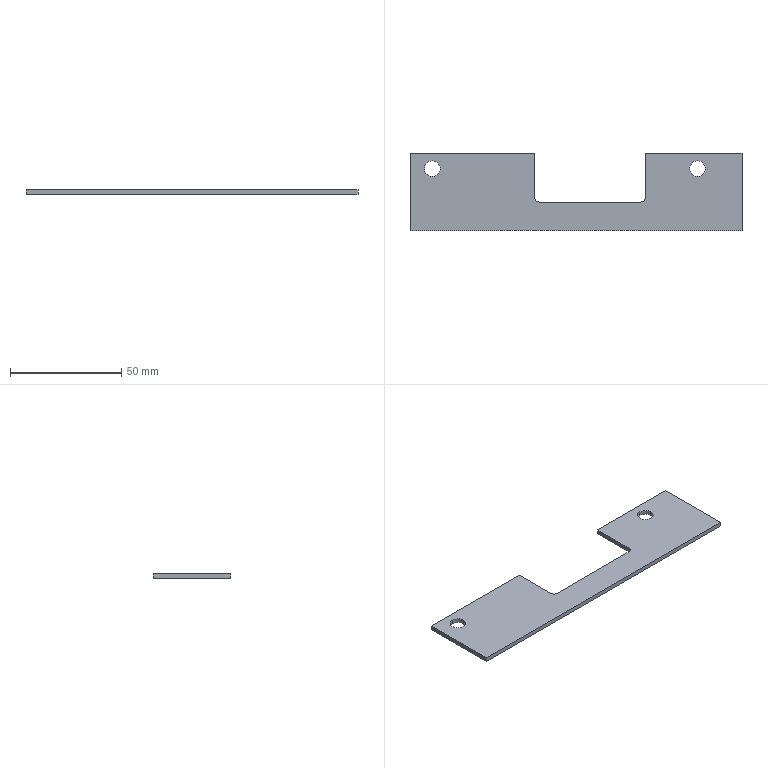Part | STEP file | 1_id638_x_t | 1 solid | 16 faces | box 149 x 35 x 2 mm | volume 8095 mm3 | plane 10 | cylinder 6 | commonest cylinder face diameters 7 x4 4 x2
STEP:
#1=CARTESIAN_POINT('',(0.,0.,0.));
#2=DIRECTION('',(0.,0.,1.));
#3=DIRECTION('',(1.,0.,0.));
#4=AXIS2_PLACEMENT_3D('',#1,#2,#3);
#5=CARTESIAN_POINT('',(650.204,237.475,-88.));
#6=VERTEX_POINT('',#5);
#7=CARTESIAN_POINT('',(648.204,235.475,-88.));
#8=VERTEX_POINT('',#7);
#9=CARTESIAN_POINT('',(648.204,237.475,-88.));
#10=DIRECTION('',(0.,0.,-1.));
#11=DIRECTION('',(1.,0.,0.));
#12=AXIS2_PLACEMENT_3D('',#9,#10,#11);
#13=CIRCLE('',#12,2.);
#14=CARTESIAN_POINT('',(499.55,257.475,-88.));
#15=DIRECTION('',(0.,0.,1.));
#16=DIRECTION('',(0.,1.,0.));
#17=AXIS2_PLACEMENT_3D('',#14,#15,#16);
#18=PLANE('',#17);
#19=CARTESIAN_POINT('',(-20.,-150.654));
#20=CARTESIAN_POINT('',(-23.464,-150.654));
#21=CARTESIAN_POINT('',(-21.732,-147.654));
#22=CARTESIAN_POINT('',(-20.,-144.654));
#23=CARTESIAN_POINT('',(-18.268,-147.654));
#24=CARTESIAN_POINT('',(-16.536,-150.654));
#25=CARTESIAN_POINT('',(-20.,-150.654));
#26=(BOUNDED_CURVE()B_SPLINE_CURVE(2,(#19,#20,#21,#22,#23,#24,#25),.UNSPECIFIED.,.T.,.F.)B_SPLINE_CURVE_WITH_KNOTS((1,2,2,2,2,1),(-2.094,0.,2.094,4.189,6.283,8.378),.UNSPECIFIED.)CURVE()GEOMETRIC_REPRESENTATION_ITEM()RATIONAL_B_SPLINE_CURVE((1.,0.5,1.,0.5,1.,0.5,1.))REPRESENTATION_ITEM(''));
#27=(GEOMETRIC_REPRESENTATION_CONTEXT(2)PARAMETRIC_REPRESENTATION_CONTEXT()REPRESENTATION_CONTEXT('',''));
#28=DEFINITIONAL_REPRESENTATION('',(#26),#27);
#29=PCURVE('',#18,#28);
#30=CARTESIAN_POINT('',(648.204,237.475,-92.));
#31=DIRECTION('',(0.,0.,-1.));
#32=DIRECTION('',(0.,1.,0.));
#33=AXIS2_PLACEMENT_3D('',#30,#31,#32);
#34=CYLINDRICAL_SURFACE('',#33,2.);
#35=CARTESIAN_POINT('',(1.571,-4.));
#36=DIRECTION('',(1.,0.));
#37=VECTOR('',#36,1.);
#38=LINE('',#35,#37);
#39=(GEOMETRIC_REPRESENTATION_CONTEXT(2)PARAMETRIC_REPRESENTATION_CONTEXT()REPRESENTATION_CONTEXT('',''));
#40=DEFINITIONAL_REPRESENTATION('',(#38),#39);
#41=PCURVE('',#34,#40);
#42=SURFACE_CURVE('',#13,(#29,#41),.PCURVE_S1.);
#43=EDGE_CURVE('',#6,#8,#42,.T.);
#44=ORIENTED_EDGE('',*,*,#43,.T.);
#45=CARTESIAN_POINT('',(602.55,235.475,-88.));
#46=VERTEX_POINT('',#45);
#47=CARTESIAN_POINT('',(648.204,235.475,-88.));
#48=DIRECTION('',(-1.,0.,0.));
#49=VECTOR('',#48,1.);
#50=LINE('',#47,#49);
#51=CARTESIAN_POINT('',(-22.,-148.654));
#52=DIRECTION('',(0.,1.));
#53=VECTOR('',#52,1.);
#54=LINE('',#51,#53);
#55=(GEOMETRIC_REPRESENTATION_CONTEXT(2)PARAMETRIC_REPRESENTATION_CONTEXT()REPRESENTATION_CONTEXT('',''));
#56=DEFINITIONAL_REPRESENTATION('',(#54),#55);
#57=PCURVE('',#18,#56);
#58=CARTESIAN_POINT('',(629.402,235.475,-92.));
#59=DIRECTION('',(0.,-1.,0.));
#60=DIRECTION('',(0.,0.,-1.));
#61=AXIS2_PLACEMENT_3D('',#58,#59,#60);
#62=PLANE('',#61);
#63=CARTESIAN_POINT('',(-4.,18.802));
#64=DIRECTION('',(0.,-1.));
#65=VECTOR('',#64,1.);
#66=LINE('',#63,#65);
#67=(GEOMETRIC_REPRESENTATION_CONTEXT(2)PARAMETRIC_REPRESENTATION_CONTEXT()REPRESENTATION_CONTEXT('',''));
#68=DEFINITIONAL_REPRESENTATION('',(#66),#67);
#69=PCURVE('',#62,#68);
#70=SURFACE_CURVE('',#50,(#57,#69),.PCURVE_S1.);
#71=EDGE_CURVE('',#8,#46,#70,.T.);
#72=ORIENTED_EDGE('',*,*,#71,.T.);
#73=CARTESIAN_POINT('',(600.55,237.475,-88.));
#74=VERTEX_POINT('',#73);
#75=CARTESIAN_POINT('',(602.55,237.475,-88.));
#76=DIRECTION('',(0.,0.,-1.));
#77=DIRECTION('',(0.,-1.,0.));
#78=AXIS2_PLACEMENT_3D('',#75,#76,#77);
#79=CIRCLE('',#78,2.);
#80=CARTESIAN_POINT('',(-22.,-103.));
#81=CARTESIAN_POINT('',(-22.,-99.536));
#82=CARTESIAN_POINT('',(-19.,-101.268));
#83=CARTESIAN_POINT('',(-16.,-103.));
#84=CARTESIAN_POINT('',(-19.,-104.732));
#85=CARTESIAN_POINT('',(-22.,-106.464));
#86=CARTESIAN_POINT('',(-22.,-103.));
#87=(BOUNDED_CURVE()B_SPLINE_CURVE(2,(#80,#81,#82,#83,#84,#85,#86),.UNSPECIFIED.,.T.,.F.)B_SPLINE_CURVE_WITH_KNOTS((1,2,2,2,2,1),(-2.094,0.,2.094,4.189,6.283,8.378),.UNSPECIFIED.)CURVE()GEOMETRIC_REPRESENTATION_ITEM()RATIONAL_B_SPLINE_CURVE((1.,0.5,1.,0.5,1.,0.5,1.))REPRESENTATION_ITEM(''));
#88=(GEOMETRIC_REPRESENTATION_CONTEXT(2)PARAMETRIC_REPRESENTATION_CONTEXT()REPRESENTATION_CONTEXT('',''));
#89=DEFINITIONAL_REPRESENTATION('',(#87),#88);
#90=PCURVE('',#18,#89);
#91=CARTESIAN_POINT('',(602.55,237.475,-92.));
#92=DIRECTION('',(0.,0.,-1.));
#93=DIRECTION('',(0.,1.,0.));
#94=AXIS2_PLACEMENT_3D('',#91,#92,#93);
#95=CYLINDRICAL_SURFACE('',#94,2.);
#96=CARTESIAN_POINT('',(3.142,-4.));
#97=DIRECTION('',(1.,0.));
#98=VECTOR('',#97,1.);
#99=LINE('',#96,#98);
#100=(GEOMETRIC_REPRESENTATION_CONTEXT(2)PARAMETRIC_REPRESENTATION_CONTEXT()REPRESENTATION_CONTEXT('',''));
#101=DEFINITIONAL_REPRESENTATION('',(#99),#100);
#102=PCURVE('',#95,#101);
#103=SURFACE_CURVE('',#79,(#90,#102),.PCURVE_S1.);
#104=EDGE_CURVE('',#46,#74,#103,.T.);
#105=ORIENTED_EDGE('',*,*,#104,.T.);
#106=CARTESIAN_POINT('',(600.55,257.475,-88.));
#107=VERTEX_POINT('',#106);
#108=CARTESIAN_POINT('',(600.55,237.475,-88.));
#109=DIRECTION('',(0.,1.,0.));
#110=VECTOR('',#109,1.);
#111=LINE('',#108,#110);
#112=CARTESIAN_POINT('',(-20.,-101.));
#113=DIRECTION('',(1.,0.));
#114=VECTOR('',#113,1.);
#115=LINE('',#112,#114);
#116=(GEOMETRIC_REPRESENTATION_CONTEXT(2)PARAMETRIC_REPRESENTATION_CONTEXT()REPRESENTATION_CONTEXT('',''));
#117=DEFINITIONAL_REPRESENTATION('',(#115),#116);
#118=PCURVE('',#18,#117);
#119=CARTESIAN_POINT('',(600.55,253.588,-92.));
#120=DIRECTION('',(-1.,0.,0.));
#121=DIRECTION('',(0.,0.,-1.));
#122=AXIS2_PLACEMENT_3D('',#119,#120,#121);
#123=PLANE('',#122);
#124=CARTESIAN_POINT('',(-4.,16.113));
#125=DIRECTION('',(0.,-1.));
#126=VECTOR('',#125,1.);
#127=LINE('',#124,#126);
#128=(GEOMETRIC_REPRESENTATION_CONTEXT(2)PARAMETRIC_REPRESENTATION_CONTEXT()REPRESENTATION_CONTEXT('',''));
#129=DEFINITIONAL_REPRESENTATION('',(#127),#128);
#130=PCURVE('',#123,#129);
#131=SURFACE_CURVE('',#111,(#118,#130),.PCURVE_S1.);
#132=EDGE_CURVE('',#74,#107,#131,.T.);
#133=ORIENTED_EDGE('',*,*,#132,.T.);
#134=CARTESIAN_POINT('',(544.55,257.475,-88.));
#135=VERTEX_POINT('',#134);
#136=CARTESIAN_POINT('',(544.55,257.475,-88.));
#137=DIRECTION('',(1.,0.,0.));
#138=VECTOR('',#137,1.);
#139=LINE('',#136,#138);
#140=CARTESIAN_POINT('',(0.,-45.));
#141=DIRECTION('',(0.,-1.));
#142=VECTOR('',#141,1.);
#143=LINE('',#140,#142);
#144=(GEOMETRIC_REPRESENTATION_CONTEXT(2)PARAMETRIC_REPRESENTATION_CONTEXT()REPRESENTATION_CONTEXT('',''));
#145=DEFINITIONAL_REPRESENTATION('',(#143),#144);
#146=PCURVE('',#18,#145);
#147=CARTESIAN_POINT('',(744.55,257.475,-88.));
#148=DIRECTION('',(0.,-1.,0.));
#149=DIRECTION('',(1.,0.,0.));
#150=AXIS2_PLACEMENT_3D('',#147,#148,#149);
#151=PLANE('',#150);
#152=CARTESIAN_POINT('',(-200.,0.));
#153=DIRECTION('',(1.,0.));
#154=VECTOR('',#153,1.);
#155=LINE('',#152,#154);
#156=(GEOMETRIC_REPRESENTATION_CONTEXT(2)PARAMETRIC_REPRESENTATION_CONTEXT()REPRESENTATION_CONTEXT('',''));
#157=DEFINITIONAL_REPRESENTATION('',(#155),#156);
#158=PCURVE('',#151,#157);
#159=SURFACE_CURVE('',#139,(#146,#158),.PCURVE_S1.);
#160=EDGE_CURVE('',#135,#107,#159,.T.);
#161=ORIENTED_EDGE('',*,*,#160,.F.);
#162=CARTESIAN_POINT('',(544.55,222.475,-88.));
#163=VERTEX_POINT('',#162);
#164=CARTESIAN_POINT('',(544.55,222.475,-88.));
#165=DIRECTION('',(0.,1.,0.));
#166=VECTOR('',#165,1.);
#167=LINE('',#164,#166);
#168=CARTESIAN_POINT('',(-35.,-45.));
#169=DIRECTION('',(1.,0.));
#170=VECTOR('',#169,1.);
#171=LINE('',#168,#170);
#172=(GEOMETRIC_REPRESENTATION_CONTEXT(2)PARAMETRIC_REPRESENTATION_CONTEXT()REPRESENTATION_CONTEXT('',''));
#173=DEFINITIONAL_REPRESENTATION('',(#171),#172);
#174=PCURVE('',#18,#173);
#175=CARTESIAN_POINT('',(544.55,257.475,-88.));
#176=DIRECTION('',(1.,0.,0.));
#177=DIRECTION('',(0.,0.,1.));
#178=AXIS2_PLACEMENT_3D('',#175,#176,#177);
#179=PLANE('',#178);
#180=CARTESIAN_POINT('',(0.,35.));
#181=DIRECTION('',(0.,-1.));
#182=VECTOR('',#181,1.);
#183=LINE('',#180,#182);
#184=(GEOMETRIC_REPRESENTATION_CONTEXT(2)PARAMETRIC_REPRESENTATION_CONTEXT()REPRESENTATION_CONTEXT('',''));
#185=DEFINITIONAL_REPRESENTATION('',(#183),#184);
#186=PCURVE('',#179,#185);
#187=SURFACE_CURVE('',#167,(#174,#186),.PCURVE_S1.);
#188=EDGE_CURVE('',#163,#135,#187,.T.);
#189=ORIENTED_EDGE('',*,*,#188,.F.);
#190=CARTESIAN_POINT('',(693.55,222.475,-88.));
#191=VERTEX_POINT('',#190);
#192=CARTESIAN_POINT('',(693.55,222.475,-88.));
#193=DIRECTION('',(-1.,0.,0.));
#194=VECTOR('',#193,1.);
#195=LINE('',#192,#194);
#196=CARTESIAN_POINT('',(-35.,-194.));
#197=DIRECTION('',(0.,1.));
#198=VECTOR('',#197,1.);
#199=LINE('',#196,#198);
#200=(GEOMETRIC_REPRESENTATION_CONTEXT(2)PARAMETRIC_REPRESENTATION_CONTEXT()REPRESENTATION_CONTEXT('',''));
#201=DEFINITIONAL_REPRESENTATION('',(#199),#200);
#202=PCURVE('',#18,#201);
#203=CARTESIAN_POINT('',(629.402,222.475,-52.5));
#204=DIRECTION('',(0.,-1.,0.));
#205=DIRECTION('',(0.,0.,-1.));
#206=AXIS2_PLACEMENT_3D('',#203,#204,#205);
#207=PLANE('',#206);
#208=CARTESIAN_POINT('',(35.5,64.148));
#209=DIRECTION('',(0.,-1.));
#210=VECTOR('',#209,1.);
#211=LINE('',#208,#210);
#212=(GEOMETRIC_REPRESENTATION_CONTEXT(2)PARAMETRIC_REPRESENTATION_CONTEXT()REPRESENTATION_CONTEXT('',''));
#213=DEFINITIONAL_REPRESENTATION('',(#211),#212);
#214=PCURVE('',#207,#213);
#215=SURFACE_CURVE('',#195,(#202,#214),.PCURVE_S1.);
#216=EDGE_CURVE('',#191,#163,#215,.T.);
#217=ORIENTED_EDGE('',*,*,#216,.F.);
#218=CARTESIAN_POINT('',(693.55,257.475,-88.));
#219=VERTEX_POINT('',#218);
#220=CARTESIAN_POINT('',(693.55,257.475,-88.));
#221=DIRECTION('',(0.,-1.,0.));
#222=VECTOR('',#221,1.);
#223=LINE('',#220,#222);
#224=CARTESIAN_POINT('',(0.,-194.));
#225=DIRECTION('',(-1.,0.));
#226=VECTOR('',#225,1.);
#227=LINE('',#224,#226);
#228=(GEOMETRIC_REPRESENTATION_CONTEXT(2)PARAMETRIC_REPRESENTATION_CONTEXT()REPRESENTATION_CONTEXT('',''));
#229=DEFINITIONAL_REPRESENTATION('',(#227),#228);
#230=PCURVE('',#18,#229);
#231=CARTESIAN_POINT('',(693.55,212.475,-88.));
#232=DIRECTION('',(-1.,0.,0.));
#233=DIRECTION('',(0.,0.,-1.));
#234=AXIS2_PLACEMENT_3D('',#231,#232,#233);
#235=PLANE('',#234);
#236=CARTESIAN_POINT('',(0.,-45.));
#237=DIRECTION('',(0.,1.));
#238=VECTOR('',#237,1.);
#239=LINE('',#236,#238);
#240=(GEOMETRIC_REPRESENTATION_CONTEXT(2)PARAMETRIC_REPRESENTATION_CONTEXT()REPRESENTATION_CONTEXT('',''));
#241=DEFINITIONAL_REPRESENTATION('',(#239),#240);
#242=PCURVE('',#235,#241);
#243=SURFACE_CURVE('',#223,(#230,#242),.PCURVE_S1.);
#244=EDGE_CURVE('',#219,#191,#243,.T.);
#245=ORIENTED_EDGE('',*,*,#244,.F.);
#246=CARTESIAN_POINT('',(650.204,257.475,-88.));
#247=VERTEX_POINT('',#246);
#248=CARTESIAN_POINT('',(650.204,257.475,-88.));
#249=DIRECTION('',(1.,0.,0.));
#250=VECTOR('',#249,1.);
#251=LINE('',#248,#250);
#252=CARTESIAN_POINT('',(0.,-150.654));
#253=DIRECTION('',(0.,-1.));
#254=VECTOR('',#253,1.);
#255=LINE('',#252,#254);
#256=(GEOMETRIC_REPRESENTATION_CONTEXT(2)PARAMETRIC_REPRESENTATION_CONTEXT()REPRESENTATION_CONTEXT('',''));
#257=DEFINITIONAL_REPRESENTATION('',(#255),#256);
#258=PCURVE('',#18,#257);
#259=CARTESIAN_POINT('',(744.55,257.475,-88.));
#260=DIRECTION('',(0.,-1.,0.));
#261=DIRECTION('',(1.,0.,0.));
#262=AXIS2_PLACEMENT_3D('',#259,#260,#261);
#263=PLANE('',#262);
#264=CARTESIAN_POINT('',(-94.346,0.));
#265=DIRECTION('',(1.,0.));
#266=VECTOR('',#265,1.);
#267=LINE('',#264,#266);
#268=(GEOMETRIC_REPRESENTATION_CONTEXT(2)PARAMETRIC_REPRESENTATION_CONTEXT()REPRESENTATION_CONTEXT('',''));
#269=DEFINITIONAL_REPRESENTATION('',(#267),#268);
#270=PCURVE('',#263,#269);
#271=SURFACE_CURVE('',#251,(#258,#270),.PCURVE_S1.);
#272=EDGE_CURVE('',#247,#219,#271,.T.);
#273=ORIENTED_EDGE('',*,*,#272,.F.);
#274=CARTESIAN_POINT('',(650.204,257.475,-88.));
#275=DIRECTION('',(0.,-1.,0.));
#276=VECTOR('',#275,1.);
#277=LINE('',#274,#276);
#278=CARTESIAN_POINT('',(0.,-150.654));
#279=DIRECTION('',(-1.,0.));
#280=VECTOR('',#279,1.);
#281=LINE('',#278,#280);
#282=(GEOMETRIC_REPRESENTATION_CONTEXT(2)PARAMETRIC_REPRESENTATION_CONTEXT()REPRESENTATION_CONTEXT('',''));
#283=DEFINITIONAL_REPRESENTATION('',(#281),#282);
#284=PCURVE('',#18,#283);
#285=CARTESIAN_POINT('',(650.204,253.588,-92.));
#286=DIRECTION('',(1.,0.,0.));
#287=DIRECTION('',(0.,0.,1.));
#288=AXIS2_PLACEMENT_3D('',#285,#286,#287);
#289=PLANE('',#288);
#290=CARTESIAN_POINT('',(4.,-3.888));
#291=DIRECTION('',(0.,1.));
#292=VECTOR('',#291,1.);
#293=LINE('',#290,#292);
#294=(GEOMETRIC_REPRESENTATION_CONTEXT(2)PARAMETRIC_REPRESENTATION_CONTEXT()REPRESENTATION_CONTEXT('',''));
#295=DEFINITIONAL_REPRESENTATION('',(#293),#294);
#296=PCURVE('',#289,#295);
#297=SURFACE_CURVE('',#277,(#284,#296),.PCURVE_S1.);
#298=EDGE_CURVE('',#247,#6,#297,.T.);
#299=ORIENTED_EDGE('',*,*,#298,.T.);
#300=EDGE_LOOP('',(#44,#72,#105,#133,#161,#189,#217,#245,#273,#299));
#301=FACE_BOUND('',#300,.T.);
#302=CARTESIAN_POINT('',(673.55,246.975,-88.));
#303=VERTEX_POINT('',#302);
#304=CARTESIAN_POINT('',(673.55,253.975,-88.));
#305=VERTEX_POINT('',#304);
#306=CARTESIAN_POINT('',(673.55,250.475,-88.));
#307=DIRECTION('',(0.,0.,-1.));
#308=DIRECTION('',(0.,-1.,0.));
#309=AXIS2_PLACEMENT_3D('',#306,#307,#308);
#310=CIRCLE('',#309,3.5);
#311=CARTESIAN_POINT('',(-10.5,-174.));
#312=CARTESIAN_POINT('',(-10.5,-167.938));
#313=CARTESIAN_POINT('',(-5.25,-170.969));
#314=CARTESIAN_POINT('',(0.,-174.));
#315=CARTESIAN_POINT('',(-5.25,-177.031));
#316=CARTESIAN_POINT('',(-10.5,-180.062));
#317=CARTESIAN_POINT('',(-10.5,-174.));
#318=(BOUNDED_CURVE()B_SPLINE_CURVE(2,(#311,#312,#313,#314,#315,#316,#317),.UNSPECIFIED.,.T.,.F.)B_SPLINE_CURVE_WITH_KNOTS((1,2,2,2,2,1),(-2.094,0.,2.094,4.189,6.283,8.378),.UNSPECIFIED.)CURVE()GEOMETRIC_REPRESENTATION_ITEM()RATIONAL_B_SPLINE_CURVE((1.,0.5,1.,0.5,1.,0.5,1.))REPRESENTATION_ITEM(''));
#319=(GEOMETRIC_REPRESENTATION_CONTEXT(2)PARAMETRIC_REPRESENTATION_CONTEXT()REPRESENTATION_CONTEXT('',''));
#320=DEFINITIONAL_REPRESENTATION('',(#318),#319);
#321=PCURVE('',#18,#320);
#322=CARTESIAN_POINT('',(673.55,250.475,-88.));
#323=DIRECTION('',(0.,0.,-1.));
#324=DIRECTION('',(0.,-1.,0.));
#325=AXIS2_PLACEMENT_3D('',#322,#323,#324);
#326=CYLINDRICAL_SURFACE('',#325,3.5);
#327=CARTESIAN_POINT('',(0.,0.));
#328=DIRECTION('',(1.,0.));
#329=VECTOR('',#328,1.);
#330=LINE('',#327,#329);
#331=(GEOMETRIC_REPRESENTATION_CONTEXT(2)PARAMETRIC_REPRESENTATION_CONTEXT()REPRESENTATION_CONTEXT('',''));
#332=DEFINITIONAL_REPRESENTATION('',(#330),#331);
#333=PCURVE('',#326,#332);
#334=SURFACE_CURVE('',#310,(#321,#333),.PCURVE_S1.);
#335=EDGE_CURVE('',#303,#305,#334,.T.);
#336=ORIENTED_EDGE('',*,*,#335,.T.);
#337=CARTESIAN_POINT('',(673.55,250.475,-88.));
#338=DIRECTION('',(0.,0.,-1.));
#339=DIRECTION('',(0.,1.,0.));
#340=AXIS2_PLACEMENT_3D('',#337,#338,#339);
#341=CIRCLE('',#340,3.5);
#342=CARTESIAN_POINT('',(-3.5,-174.));
#343=CARTESIAN_POINT('',(-3.5,-180.062));
#344=CARTESIAN_POINT('',(-8.75,-177.031));
#345=CARTESIAN_POINT('',(-14.,-174.));
#346=CARTESIAN_POINT('',(-8.75,-170.969));
#347=CARTESIAN_POINT('',(-3.5,-167.938));
#348=CARTESIAN_POINT('',(-3.5,-174.));
#349=(BOUNDED_CURVE()B_SPLINE_CURVE(2,(#342,#343,#344,#345,#346,#347,#348),.UNSPECIFIED.,.T.,.F.)B_SPLINE_CURVE_WITH_KNOTS((1,2,2,2,2,1),(-2.094,0.,2.094,4.189,6.283,8.378),.UNSPECIFIED.)CURVE()GEOMETRIC_REPRESENTATION_ITEM()RATIONAL_B_SPLINE_CURVE((1.,0.5,1.,0.5,1.,0.5,1.))REPRESENTATION_ITEM(''));
#350=(GEOMETRIC_REPRESENTATION_CONTEXT(2)PARAMETRIC_REPRESENTATION_CONTEXT()REPRESENTATION_CONTEXT('',''));
#351=DEFINITIONAL_REPRESENTATION('',(#349),#350);
#352=PCURVE('',#18,#351);
#353=CARTESIAN_POINT('',(673.55,250.475,-88.));
#354=DIRECTION('',(0.,0.,-1.));
#355=DIRECTION('',(0.,-1.,0.));
#356=AXIS2_PLACEMENT_3D('',#353,#354,#355);
#357=CYLINDRICAL_SURFACE('',#356,3.5);
#358=CARTESIAN_POINT('',(3.142,0.));
#359=DIRECTION('',(1.,0.));
#360=VECTOR('',#359,1.);
#361=LINE('',#358,#360);
#362=(GEOMETRIC_REPRESENTATION_CONTEXT(2)PARAMETRIC_REPRESENTATION_CONTEXT()REPRESENTATION_CONTEXT('',''));
#363=DEFINITIONAL_REPRESENTATION('',(#361),#362);
#364=PCURVE('',#357,#363);
#365=SURFACE_CURVE('',#341,(#352,#364),.PCURVE_S1.);
#366=EDGE_CURVE('',#305,#303,#365,.T.);
#367=ORIENTED_EDGE('',*,*,#366,.T.);
#368=EDGE_LOOP('',(#336,#367));
#369=FACE_BOUND('',#368,.T.);
#370=CARTESIAN_POINT('',(554.55,246.975,-88.));
#371=VERTEX_POINT('',#370);
#372=CARTESIAN_POINT('',(554.55,253.975,-88.));
#373=VERTEX_POINT('',#372);
#374=CARTESIAN_POINT('',(554.55,250.475,-88.));
#375=DIRECTION('',(0.,0.,-1.));
#376=DIRECTION('',(0.,-1.,0.));
#377=AXIS2_PLACEMENT_3D('',#374,#375,#376);
#378=CIRCLE('',#377,3.5);
#379=CARTESIAN_POINT('',(-10.5,-55.));
#380=CARTESIAN_POINT('',(-10.5,-48.938));
#381=CARTESIAN_POINT('',(-5.25,-51.969));
#382=CARTESIAN_POINT('',(0.,-55.));
#383=CARTESIAN_POINT('',(-5.25,-58.031));
#384=CARTESIAN_POINT('',(-10.5,-61.062));
#385=CARTESIAN_POINT('',(-10.5,-55.));
#386=(BOUNDED_CURVE()B_SPLINE_CURVE(2,(#379,#380,#381,#382,#383,#384,#385),.UNSPECIFIED.,.T.,.F.)B_SPLINE_CURVE_WITH_KNOTS((1,2,2,2,2,1),(-2.094,0.,2.094,4.189,6.283,8.378),.UNSPECIFIED.)CURVE()GEOMETRIC_REPRESENTATION_ITEM()RATIONAL_B_SPLINE_CURVE((1.,0.5,1.,0.5,1.,0.5,1.))REPRESENTATION_ITEM(''));
#387=(GEOMETRIC_REPRESENTATION_CONTEXT(2)PARAMETRIC_REPRESENTATION_CONTEXT()REPRESENTATION_CONTEXT('',''));
#388=DEFINITIONAL_REPRESENTATION('',(#386),#387);
#389=PCURVE('',#18,#388);
#390=CARTESIAN_POINT('',(554.55,250.475,-88.));
#391=DIRECTION('',(0.,0.,-1.));
#392=DIRECTION('',(0.,-1.,0.));
#393=AXIS2_PLACEMENT_3D('',#390,#391,#392);
#394=CYLINDRICAL_SURFACE('',#393,3.5);
#395=CARTESIAN_POINT('',(0.,0.));
#396=DIRECTION('',(1.,0.));
#397=VECTOR('',#396,1.);
#398=LINE('',#395,#397);
#399=(GEOMETRIC_REPRESENTATION_CONTEXT(2)PARAMETRIC_REPRESENTATION_CONTEXT()REPRESENTATION_CONTEXT('',''));
#400=DEFINITIONAL_REPRESENTATION('',(#398),#399);
#401=PCURVE('',#394,#400);
#402=SURFACE_CURVE('',#378,(#389,#401),.PCURVE_S1.);
#403=EDGE_CURVE('',#371,#373,#402,.T.);
#404=ORIENTED_EDGE('',*,*,#403,.T.);
#405=CARTESIAN_POINT('',(554.55,250.475,-88.));
#406=DIRECTION('',(0.,0.,-1.));
#407=DIRECTION('',(0.,1.,0.));
#408=AXIS2_PLACEMENT_3D('',#405,#406,#407);
#409=CIRCLE('',#408,3.5);
#410=CARTESIAN_POINT('',(-3.5,-55.));
#411=CARTESIAN_POINT('',(-3.5,-61.062));
#412=CARTESIAN_POINT('',(-8.75,-58.031));
#413=CARTESIAN_POINT('',(-14.,-55.));
#414=CARTESIAN_POINT('',(-8.75,-51.969));
#415=CARTESIAN_POINT('',(-3.5,-48.938));
#416=CARTESIAN_POINT('',(-3.5,-55.));
#417=(BOUNDED_CURVE()B_SPLINE_CURVE(2,(#410,#411,#412,#413,#414,#415,#416),.UNSPECIFIED.,.T.,.F.)B_SPLINE_CURVE_WITH_KNOTS((1,2,2,2,2,1),(-2.094,0.,2.094,4.189,6.283,8.378),.UNSPECIFIED.)CURVE()GEOMETRIC_REPRESENTATION_ITEM()RATIONAL_B_SPLINE_CURVE((1.,0.5,1.,0.5,1.,0.5,1.))REPRESENTATION_ITEM(''));
#418=(GEOMETRIC_REPRESENTATION_CONTEXT(2)PARAMETRIC_REPRESENTATION_CONTEXT()REPRESENTATION_CONTEXT('',''));
#419=DEFINITIONAL_REPRESENTATION('',(#417),#418);
#420=PCURVE('',#18,#419);
#421=CARTESIAN_POINT('',(554.55,250.475,-88.));
#422=DIRECTION('',(0.,0.,-1.));
#423=DIRECTION('',(0.,-1.,0.));
#424=AXIS2_PLACEMENT_3D('',#421,#422,#423);
#425=CYLINDRICAL_SURFACE('',#424,3.5);
#426=CARTESIAN_POINT('',(3.142,0.));
#427=DIRECTION('',(1.,0.));
#428=VECTOR('',#427,1.);
#429=LINE('',#426,#428);
#430=(GEOMETRIC_REPRESENTATION_CONTEXT(2)PARAMETRIC_REPRESENTATION_CONTEXT()REPRESENTATION_CONTEXT('',''));
#431=DEFINITIONAL_REPRESENTATION('',(#429),#430);
#432=PCURVE('',#425,#431);
#433=SURFACE_CURVE('',#409,(#420,#432),.PCURVE_S1.);
#434=EDGE_CURVE('',#373,#371,#433,.T.);
#435=ORIENTED_EDGE('',*,*,#434,.T.);
#436=EDGE_LOOP('',(#404,#435));
#437=FACE_BOUND('',#436,.T.);
#438=ADVANCED_FACE('',(#301,#369,#437),#18,.T.);
#439=CARTESIAN_POINT('',(650.204,237.475,-90.));
#440=VERTEX_POINT('',#439);
#441=CARTESIAN_POINT('',(650.204,237.475,-88.));
#442=DIRECTION('',(0.,0.,-1.));
#443=VECTOR('',#442,1.);
#444=LINE('',#441,#443);
#445=CARTESIAN_POINT('',(4.,16.113));
#446=DIRECTION('',(-1.,0.));
#447=VECTOR('',#446,1.);
#448=LINE('',#445,#447);
#449=(GEOMETRIC_REPRESENTATION_CONTEXT(2)PARAMETRIC_REPRESENTATION_CONTEXT()REPRESENTATION_CONTEXT('',''));
#450=DEFINITIONAL_REPRESENTATION('',(#448),#449);
#451=PCURVE('',#289,#450);
#452=CARTESIAN_POINT('',(1.571,-4.));
#453=DIRECTION('',(0.,1.));
#454=VECTOR('',#453,1.);
#455=LINE('',#452,#454);
#456=(GEOMETRIC_REPRESENTATION_CONTEXT(2)PARAMETRIC_REPRESENTATION_CONTEXT()REPRESENTATION_CONTEXT('',''));
#457=DEFINITIONAL_REPRESENTATION('',(#455),#456);
#458=PCURVE('',#34,#457);
#459=SURFACE_CURVE('',#444,(#451,#458),.PCURVE_S1.);
#460=EDGE_CURVE('',#6,#440,#459,.T.);
#461=ORIENTED_EDGE('',*,*,#460,.F.);
#462=ORIENTED_EDGE('',*,*,#298,.F.);
#463=CARTESIAN_POINT('',(650.204,257.475,-90.));
#464=VERTEX_POINT('',#463);
#465=CARTESIAN_POINT('',(650.204,257.475,-88.));
#466=DIRECTION('',(0.,0.,-1.));
#467=VECTOR('',#466,1.);
#468=LINE('',#465,#467);
#469=CARTESIAN_POINT('',(4.,-3.888));
#470=DIRECTION('',(-1.,0.));
#471=VECTOR('',#470,1.);
#472=LINE('',#469,#471);
#473=(GEOMETRIC_REPRESENTATION_CONTEXT(2)PARAMETRIC_REPRESENTATION_CONTEXT()REPRESENTATION_CONTEXT('',''));
#474=DEFINITIONAL_REPRESENTATION('',(#472),#473);
#475=PCURVE('',#289,#474);
#476=CARTESIAN_POINT('',(-94.346,0.));
#477=DIRECTION('',(0.,-1.));
#478=VECTOR('',#477,1.);
#479=LINE('',#476,#478);
#480=(GEOMETRIC_REPRESENTATION_CONTEXT(2)PARAMETRIC_REPRESENTATION_CONTEXT()REPRESENTATION_CONTEXT('',''));
#481=DEFINITIONAL_REPRESENTATION('',(#479),#480);
#482=PCURVE('',#263,#481);
#483=SURFACE_CURVE('',#468,(#475,#482),.PCURVE_S1.);
#484=EDGE_CURVE('',#247,#464,#483,.T.);
#485=ORIENTED_EDGE('',*,*,#484,.T.);
#486=CARTESIAN_POINT('',(650.204,257.475,-90.));
#487=DIRECTION('',(0.,-1.,0.));
#488=VECTOR('',#487,1.);
#489=LINE('',#486,#488);
#490=CARTESIAN_POINT('',(2.,-3.888));
#491=DIRECTION('',(0.,1.));
#492=VECTOR('',#491,1.);
#493=LINE('',#490,#492);
#494=(GEOMETRIC_REPRESENTATION_CONTEXT(2)PARAMETRIC_REPRESENTATION_CONTEXT()REPRESENTATION_CONTEXT('',''));
#495=DEFINITIONAL_REPRESENTATION('',(#493),#494);
#496=PCURVE('',#289,#495);
#497=CARTESIAN_POINT('',(499.55,257.475,-90.));
#498=DIRECTION('',(0.,0.,1.));
#499=DIRECTION('',(0.,1.,0.));
#500=AXIS2_PLACEMENT_3D('',#497,#498,#499);
#501=PLANE('',#500);
#502=CARTESIAN_POINT('',(0.,-150.654));
#503=DIRECTION('',(-1.,0.));
#504=VECTOR('',#503,1.);
#505=LINE('',#502,#504);
#506=(GEOMETRIC_REPRESENTATION_CONTEXT(2)PARAMETRIC_REPRESENTATION_CONTEXT()REPRESENTATION_CONTEXT('',''));
#507=DEFINITIONAL_REPRESENTATION('',(#505),#506);
#508=PCURVE('',#501,#507);
#509=SURFACE_CURVE('',#489,(#496,#508),.PCURVE_S1.);
#510=EDGE_CURVE('',#464,#440,#509,.T.);
#511=ORIENTED_EDGE('',*,*,#510,.T.);
#512=EDGE_LOOP('',(#461,#462,#485,#511));
#513=FACE_BOUND('',#512,.T.);
#514=ADVANCED_FACE('',(#513),#289,.F.);
#515=CARTESIAN_POINT('',(600.55,237.475,-90.));
#516=VERTEX_POINT('',#515);
#517=CARTESIAN_POINT('',(602.55,235.475,-90.));
#518=VERTEX_POINT('',#517);
#519=CARTESIAN_POINT('',(602.55,237.475,-90.));
#520=DIRECTION('',(0.,0.,1.));
#521=DIRECTION('',(-1.,0.,0.));
#522=AXIS2_PLACEMENT_3D('',#519,#520,#521);
#523=CIRCLE('',#522,2.);
#524=CARTESIAN_POINT('',(-20.,-103.));
#525=DIRECTION('',(0.,1.));
#526=AXIS2_PLACEMENT_2D('',#524,#525);
#527=CIRCLE('',#526,2.);
#528=(GEOMETRIC_REPRESENTATION_CONTEXT(2)PARAMETRIC_REPRESENTATION_CONTEXT()REPRESENTATION_CONTEXT('',''));
#529=DEFINITIONAL_REPRESENTATION('',(#527),#528);
#530=PCURVE('',#501,#529);
#531=CARTESIAN_POINT('',(4.712,-2.));
#532=DIRECTION('',(-1.,0.));
#533=VECTOR('',#532,1.);
#534=LINE('',#531,#533);
#535=(GEOMETRIC_REPRESENTATION_CONTEXT(2)PARAMETRIC_REPRESENTATION_CONTEXT()REPRESENTATION_CONTEXT('',''));
#536=DEFINITIONAL_REPRESENTATION('',(#534),#535);
#537=PCURVE('',#95,#536);
#538=SURFACE_CURVE('',#523,(#530,#537),.PCURVE_S1.);
#539=EDGE_CURVE('',#516,#518,#538,.T.);
#540=ORIENTED_EDGE('',*,*,#539,.T.);
#541=CARTESIAN_POINT('',(648.204,235.475,-90.));
#542=VERTEX_POINT('',#541);
#543=CARTESIAN_POINT('',(648.204,235.475,-90.));
#544=DIRECTION('',(-1.,0.,0.));
#545=VECTOR('',#544,1.);
#546=LINE('',#543,#545);
#547=CARTESIAN_POINT('',(-22.,-148.654));
#548=DIRECTION('',(0.,1.));
#549=VECTOR('',#548,1.);
#550=LINE('',#547,#549);
#551=(GEOMETRIC_REPRESENTATION_CONTEXT(2)PARAMETRIC_REPRESENTATION_CONTEXT()REPRESENTATION_CONTEXT('',''));
#552=DEFINITIONAL_REPRESENTATION('',(#550),#551);
#553=PCURVE('',#501,#552);
#554=CARTESIAN_POINT('',(-2.,18.802));
#555=DIRECTION('',(0.,-1.));
#556=VECTOR('',#555,1.);
#557=LINE('',#554,#556);
#558=(GEOMETRIC_REPRESENTATION_CONTEXT(2)PARAMETRIC_REPRESENTATION_CONTEXT()REPRESENTATION_CONTEXT('',''));
#559=DEFINITIONAL_REPRESENTATION('',(#557),#558);
#560=PCURVE('',#62,#559);
#561=SURFACE_CURVE('',#546,(#553,#560),.PCURVE_S1.);
#562=EDGE_CURVE('',#542,#518,#561,.T.);
#563=ORIENTED_EDGE('',*,*,#562,.F.);
#564=CARTESIAN_POINT('',(648.204,237.475,-90.));
#565=DIRECTION('',(0.,0.,1.));
#566=DIRECTION('',(0.,-1.,0.));
#567=AXIS2_PLACEMENT_3D('',#564,#565,#566);
#568=CIRCLE('',#567,2.);
#569=CARTESIAN_POINT('',(-20.,-148.654));
#570=DIRECTION('',(-1.,0.));
#571=AXIS2_PLACEMENT_2D('',#569,#570);
#572=CIRCLE('',#571,2.);
#573=(GEOMETRIC_REPRESENTATION_CONTEXT(2)PARAMETRIC_REPRESENTATION_CONTEXT()REPRESENTATION_CONTEXT('',''));
#574=DEFINITIONAL_REPRESENTATION('',(#572),#573);
#575=PCURVE('',#501,#574);
#576=CARTESIAN_POINT('',(3.142,-2.));
#577=DIRECTION('',(-1.,0.));
#578=VECTOR('',#577,1.);
#579=LINE('',#576,#578);
#580=(GEOMETRIC_REPRESENTATION_CONTEXT(2)PARAMETRIC_REPRESENTATION_CONTEXT()REPRESENTATION_CONTEXT('',''));
#581=DEFINITIONAL_REPRESENTATION('',(#579),#580);
#582=PCURVE('',#34,#581);
#583=SURFACE_CURVE('',#568,(#575,#582),.PCURVE_S1.);
#584=EDGE_CURVE('',#542,#440,#583,.T.);
#585=ORIENTED_EDGE('',*,*,#584,.T.);
#586=ORIENTED_EDGE('',*,*,#510,.F.);
#587=CARTESIAN_POINT('',(693.55,257.475,-90.));
#588=VERTEX_POINT('',#587);
#589=CARTESIAN_POINT('',(650.204,257.475,-90.));
#590=DIRECTION('',(1.,0.,0.));
#591=VECTOR('',#590,1.);
#592=LINE('',#589,#591);
#593=CARTESIAN_POINT('',(0.,-150.654));
#594=DIRECTION('',(0.,-1.));
#595=VECTOR('',#594,1.);
#596=LINE('',#593,#595);
#597=(GEOMETRIC_REPRESENTATION_CONTEXT(2)PARAMETRIC_REPRESENTATION_CONTEXT()REPRESENTATION_CONTEXT('',''));
#598=DEFINITIONAL_REPRESENTATION('',(#596),#597);
#599=PCURVE('',#501,#598);
#600=CARTESIAN_POINT('',(-94.346,-2.));
#601=DIRECTION('',(1.,0.));
#602=VECTOR('',#601,1.);
#603=LINE('',#600,#602);
#604=(GEOMETRIC_REPRESENTATION_CONTEXT(2)PARAMETRIC_REPRESENTATION_CONTEXT()REPRESENTATION_CONTEXT('',''));
#605=DEFINITIONAL_REPRESENTATION('',(#603),#604);
#606=PCURVE('',#263,#605);
#607=SURFACE_CURVE('',#592,(#599,#606),.PCURVE_S1.);
#608=EDGE_CURVE('',#464,#588,#607,.T.);
#609=ORIENTED_EDGE('',*,*,#608,.T.);
#610=CARTESIAN_POINT('',(693.55,222.475,-90.));
#611=VERTEX_POINT('',#610);
#612=CARTESIAN_POINT('',(693.55,257.475,-90.));
#613=DIRECTION('',(0.,-1.,0.));
#614=VECTOR('',#613,1.);
#615=LINE('',#612,#614);
#616=CARTESIAN_POINT('',(0.,-194.));
#617=DIRECTION('',(-1.,0.));
#618=VECTOR('',#617,1.);
#619=LINE('',#616,#618);
#620=(GEOMETRIC_REPRESENTATION_CONTEXT(2)PARAMETRIC_REPRESENTATION_CONTEXT()REPRESENTATION_CONTEXT('',''));
#621=DEFINITIONAL_REPRESENTATION('',(#619),#620);
#622=PCURVE('',#501,#621);
#623=CARTESIAN_POINT('',(2.,-45.));
#624=DIRECTION('',(0.,1.));
#625=VECTOR('',#624,1.);
#626=LINE('',#623,#625);
#627=(GEOMETRIC_REPRESENTATION_CONTEXT(2)PARAMETRIC_REPRESENTATION_CONTEXT()REPRESENTATION_CONTEXT('',''));
#628=DEFINITIONAL_REPRESENTATION('',(#626),#627);
#629=PCURVE('',#235,#628);
#630=SURFACE_CURVE('',#615,(#622,#629),.PCURVE_S1.);
#631=EDGE_CURVE('',#588,#611,#630,.T.);
#632=ORIENTED_EDGE('',*,*,#631,.T.);
#633=CARTESIAN_POINT('',(544.55,222.475,-90.));
#634=VERTEX_POINT('',#633);
#635=CARTESIAN_POINT('',(693.55,222.475,-90.));
#636=DIRECTION('',(-1.,0.,0.));
#637=VECTOR('',#636,1.);
#638=LINE('',#635,#637);
#639=CARTESIAN_POINT('',(-35.,-194.));
#640=DIRECTION('',(0.,1.));
#641=VECTOR('',#640,1.);
#642=LINE('',#639,#641);
#643=(GEOMETRIC_REPRESENTATION_CONTEXT(2)PARAMETRIC_REPRESENTATION_CONTEXT()REPRESENTATION_CONTEXT('',''));
#644=DEFINITIONAL_REPRESENTATION('',(#642),#643);
#645=PCURVE('',#501,#644);
#646=CARTESIAN_POINT('',(37.5,64.148));
#647=DIRECTION('',(0.,-1.));
#648=VECTOR('',#647,1.);
#649=LINE('',#646,#648);
#650=(GEOMETRIC_REPRESENTATION_CONTEXT(2)PARAMETRIC_REPRESENTATION_CONTEXT()REPRESENTATION_CONTEXT('',''));
#651=DEFINITIONAL_REPRESENTATION('',(#649),#650);
#652=PCURVE('',#207,#651);
#653=SURFACE_CURVE('',#638,(#645,#652),.PCURVE_S1.);
#654=EDGE_CURVE('',#611,#634,#653,.T.);
#655=ORIENTED_EDGE('',*,*,#654,.T.);
#656=CARTESIAN_POINT('',(544.55,257.475,-90.));
#657=VERTEX_POINT('',#656);
#658=CARTESIAN_POINT('',(544.55,222.475,-90.));
#659=DIRECTION('',(0.,1.,0.));
#660=VECTOR('',#659,1.);
#661=LINE('',#658,#660);
#662=CARTESIAN_POINT('',(-35.,-45.));
#663=DIRECTION('',(1.,0.));
#664=VECTOR('',#663,1.);
#665=LINE('',#662,#664);
#666=(GEOMETRIC_REPRESENTATION_CONTEXT(2)PARAMETRIC_REPRESENTATION_CONTEXT()REPRESENTATION_CONTEXT('',''));
#667=DEFINITIONAL_REPRESENTATION('',(#665),#666);
#668=PCURVE('',#501,#667);
#669=CARTESIAN_POINT('',(-2.,35.));
#670=DIRECTION('',(0.,-1.));
#671=VECTOR('',#670,1.);
#672=LINE('',#669,#671);
#673=(GEOMETRIC_REPRESENTATION_CONTEXT(2)PARAMETRIC_REPRESENTATION_CONTEXT()REPRESENTATION_CONTEXT('',''));
#674=DEFINITIONAL_REPRESENTATION('',(#672),#673);
#675=PCURVE('',#179,#674);
#676=SURFACE_CURVE('',#661,(#668,#675),.PCURVE_S1.);
#677=EDGE_CURVE('',#634,#657,#676,.T.);
#678=ORIENTED_EDGE('',*,*,#677,.T.);
#679=CARTESIAN_POINT('',(600.55,257.475,-90.));
#680=VERTEX_POINT('',#679);
#681=CARTESIAN_POINT('',(544.55,257.475,-90.));
#682=DIRECTION('',(1.,0.,0.));
#683=VECTOR('',#682,1.);
#684=LINE('',#681,#683);
#685=CARTESIAN_POINT('',(0.,-45.));
#686=DIRECTION('',(0.,-1.));
#687=VECTOR('',#686,1.);
#688=LINE('',#685,#687);
#689=(GEOMETRIC_REPRESENTATION_CONTEXT(2)PARAMETRIC_REPRESENTATION_CONTEXT()REPRESENTATION_CONTEXT('',''));
#690=DEFINITIONAL_REPRESENTATION('',(#688),#689);
#691=PCURVE('',#501,#690);
#692=CARTESIAN_POINT('',(-200.,-2.));
#693=DIRECTION('',(1.,0.));
#694=VECTOR('',#693,1.);
#695=LINE('',#692,#694);
#696=(GEOMETRIC_REPRESENTATION_CONTEXT(2)PARAMETRIC_REPRESENTATION_CONTEXT()REPRESENTATION_CONTEXT('',''));
#697=DEFINITIONAL_REPRESENTATION('',(#695),#696);
#698=PCURVE('',#151,#697);
#699=SURFACE_CURVE('',#684,(#691,#698),.PCURVE_S1.);
#700=EDGE_CURVE('',#657,#680,#699,.T.);
#701=ORIENTED_EDGE('',*,*,#700,.T.);
#702=CARTESIAN_POINT('',(600.55,237.475,-90.));
#703=DIRECTION('',(0.,1.,0.));
#704=VECTOR('',#703,1.);
#705=LINE('',#702,#704);
#706=CARTESIAN_POINT('',(-20.,-101.));
#707=DIRECTION('',(1.,0.));
#708=VECTOR('',#707,1.);
#709=LINE('',#706,#708);
#710=(GEOMETRIC_REPRESENTATION_CONTEXT(2)PARAMETRIC_REPRESENTATION_CONTEXT()REPRESENTATION_CONTEXT('',''));
#711=DEFINITIONAL_REPRESENTATION('',(#709),#710);
#712=PCURVE('',#501,#711);
#713=CARTESIAN_POINT('',(-2.,16.113));
#714=DIRECTION('',(0.,-1.));
#715=VECTOR('',#714,1.);
#716=LINE('',#713,#715);
#717=(GEOMETRIC_REPRESENTATION_CONTEXT(2)PARAMETRIC_REPRESENTATION_CONTEXT()REPRESENTATION_CONTEXT('',''));
#718=DEFINITIONAL_REPRESENTATION('',(#716),#717);
#719=PCURVE('',#123,#718);
#720=SURFACE_CURVE('',#705,(#712,#719),.PCURVE_S1.);
#721=EDGE_CURVE('',#516,#680,#720,.T.);
#722=ORIENTED_EDGE('',*,*,#721,.F.);
#723=EDGE_LOOP('',(#540,#563,#585,#586,#609,#632,#655,#678,#701,#722));
#724=FACE_BOUND('',#723,.T.);
#725=CARTESIAN_POINT('',(554.55,246.975,-90.));
#726=VERTEX_POINT('',#725);
#727=CARTESIAN_POINT('',(554.55,253.975,-90.));
#728=VERTEX_POINT('',#727);
#729=CARTESIAN_POINT('',(554.55,250.475,-90.));
#730=DIRECTION('',(0.,0.,1.));
#731=DIRECTION('',(0.,-1.,0.));
#732=AXIS2_PLACEMENT_3D('',#729,#730,#731);
#733=CIRCLE('',#732,3.5);
#734=CARTESIAN_POINT('',(-7.,-55.));
#735=DIRECTION('',(-1.,0.));
#736=AXIS2_PLACEMENT_2D('',#734,#735);
#737=CIRCLE('',#736,3.5);
#738=(GEOMETRIC_REPRESENTATION_CONTEXT(2)PARAMETRIC_REPRESENTATION_CONTEXT()REPRESENTATION_CONTEXT('',''));
#739=DEFINITIONAL_REPRESENTATION('',(#737),#738);
#740=PCURVE('',#501,#739);
#741=CARTESIAN_POINT('',(6.283,2.));
#742=DIRECTION('',(-1.,0.));
#743=VECTOR('',#742,1.);
#744=LINE('',#741,#743);
#745=(GEOMETRIC_REPRESENTATION_CONTEXT(2)PARAMETRIC_REPRESENTATION_CONTEXT()REPRESENTATION_CONTEXT('',''));
#746=DEFINITIONAL_REPRESENTATION('',(#744),#745);
#747=PCURVE('',#425,#746);
#748=SURFACE_CURVE('',#733,(#740,#747),.PCURVE_S1.);
#749=EDGE_CURVE('',#726,#728,#748,.T.);
#750=ORIENTED_EDGE('',*,*,#749,.T.);
#751=CARTESIAN_POINT('',(554.55,250.475,-90.));
#752=DIRECTION('',(0.,0.,1.));
#753=DIRECTION('',(0.,1.,0.));
#754=AXIS2_PLACEMENT_3D('',#751,#752,#753);
#755=CIRCLE('',#754,3.5);
#756=CARTESIAN_POINT('',(-7.,-55.));
#757=DIRECTION('',(1.,0.));
#758=AXIS2_PLACEMENT_2D('',#756,#757);
#759=CIRCLE('',#758,3.5);
#760=(GEOMETRIC_REPRESENTATION_CONTEXT(2)PARAMETRIC_REPRESENTATION_CONTEXT()REPRESENTATION_CONTEXT('',''));
#761=DEFINITIONAL_REPRESENTATION('',(#759),#760);
#762=PCURVE('',#501,#761);
#763=CARTESIAN_POINT('',(3.142,2.));
#764=DIRECTION('',(-1.,0.));
#765=VECTOR('',#764,1.);
#766=LINE('',#763,#765);
#767=(GEOMETRIC_REPRESENTATION_CONTEXT(2)PARAMETRIC_REPRESENTATION_CONTEXT()REPRESENTATION_CONTEXT('',''));
#768=DEFINITIONAL_REPRESENTATION('',(#766),#767);
#769=PCURVE('',#394,#768);
#770=SURFACE_CURVE('',#755,(#762,#769),.PCURVE_S1.);
#771=EDGE_CURVE('',#728,#726,#770,.T.);
#772=ORIENTED_EDGE('',*,*,#771,.T.);
#773=EDGE_LOOP('',(#750,#772));
#774=FACE_BOUND('',#773,.T.);
#775=CARTESIAN_POINT('',(673.55,246.975,-90.));
#776=VERTEX_POINT('',#775);
#777=CARTESIAN_POINT('',(673.55,253.975,-90.));
#778=VERTEX_POINT('',#777);
#779=CARTESIAN_POINT('',(673.55,250.475,-90.));
#780=DIRECTION('',(0.,0.,1.));
#781=DIRECTION('',(0.,-1.,0.));
#782=AXIS2_PLACEMENT_3D('',#779,#780,#781);
#783=CIRCLE('',#782,3.5);
#784=CARTESIAN_POINT('',(-7.,-174.));
#785=DIRECTION('',(-1.,0.));
#786=AXIS2_PLACEMENT_2D('',#784,#785);
#787=CIRCLE('',#786,3.5);
#788=(GEOMETRIC_REPRESENTATION_CONTEXT(2)PARAMETRIC_REPRESENTATION_CONTEXT()REPRESENTATION_CONTEXT('',''));
#789=DEFINITIONAL_REPRESENTATION('',(#787),#788);
#790=PCURVE('',#501,#789);
#791=CARTESIAN_POINT('',(6.283,2.));
#792=DIRECTION('',(-1.,0.));
#793=VECTOR('',#792,1.);
#794=LINE('',#791,#793);
#795=(GEOMETRIC_REPRESENTATION_CONTEXT(2)PARAMETRIC_REPRESENTATION_CONTEXT()REPRESENTATION_CONTEXT('',''));
#796=DEFINITIONAL_REPRESENTATION('',(#794),#795);
#797=PCURVE('',#357,#796);
#798=SURFACE_CURVE('',#783,(#790,#797),.PCURVE_S1.);
#799=EDGE_CURVE('',#776,#778,#798,.T.);
#800=ORIENTED_EDGE('',*,*,#799,.T.);
#801=CARTESIAN_POINT('',(673.55,250.475,-90.));
#802=DIRECTION('',(0.,0.,1.));
#803=DIRECTION('',(0.,1.,0.));
#804=AXIS2_PLACEMENT_3D('',#801,#802,#803);
#805=CIRCLE('',#804,3.5);
#806=CARTESIAN_POINT('',(-7.,-174.));
#807=DIRECTION('',(1.,0.));
#808=AXIS2_PLACEMENT_2D('',#806,#807);
#809=CIRCLE('',#808,3.5);
#810=(GEOMETRIC_REPRESENTATION_CONTEXT(2)PARAMETRIC_REPRESENTATION_CONTEXT()REPRESENTATION_CONTEXT('',''));
#811=DEFINITIONAL_REPRESENTATION('',(#809),#810);
#812=PCURVE('',#501,#811);
#813=CARTESIAN_POINT('',(3.142,2.));
#814=DIRECTION('',(-1.,0.));
#815=VECTOR('',#814,1.);
#816=LINE('',#813,#815);
#817=(GEOMETRIC_REPRESENTATION_CONTEXT(2)PARAMETRIC_REPRESENTATION_CONTEXT()REPRESENTATION_CONTEXT('',''));
#818=DEFINITIONAL_REPRESENTATION('',(#816),#817);
#819=PCURVE('',#326,#818);
#820=SURFACE_CURVE('',#805,(#812,#819),.PCURVE_S1.);
#821=EDGE_CURVE('',#778,#776,#820,.T.);
#822=ORIENTED_EDGE('',*,*,#821,.T.);
#823=EDGE_LOOP('',(#800,#822));
#824=FACE_BOUND('',#823,.T.);
#825=ADVANCED_FACE('',(#724,#774,#824),#501,.F.);
#826=CARTESIAN_POINT('',(600.55,237.475,-90.));
#827=DIRECTION('',(0.,0.,1.));
#828=VECTOR('',#827,1.);
#829=LINE('',#826,#828);
#830=CARTESIAN_POINT('',(-2.,16.113));
#831=DIRECTION('',(-1.,0.));
#832=VECTOR('',#831,1.);
#833=LINE('',#830,#832);
#834=(GEOMETRIC_REPRESENTATION_CONTEXT(2)PARAMETRIC_REPRESENTATION_CONTEXT()REPRESENTATION_CONTEXT('',''));
#835=DEFINITIONAL_REPRESENTATION('',(#833),#834);
#836=PCURVE('',#123,#835);
#837=CARTESIAN_POINT('',(4.712,-2.));
#838=DIRECTION('',(0.,-1.));
#839=VECTOR('',#838,1.);
#840=LINE('',#837,#839);
#841=(GEOMETRIC_REPRESENTATION_CONTEXT(2)PARAMETRIC_REPRESENTATION_CONTEXT()REPRESENTATION_CONTEXT('',''));
#842=DEFINITIONAL_REPRESENTATION('',(#840),#841);
#843=PCURVE('',#95,#842);
#844=SURFACE_CURVE('',#829,(#836,#843),.PCURVE_S1.);
#845=EDGE_CURVE('',#516,#74,#844,.T.);
#846=ORIENTED_EDGE('',*,*,#845,.F.);
#847=ORIENTED_EDGE('',*,*,#721,.T.);
#848=CARTESIAN_POINT('',(600.55,257.475,-90.));
#849=DIRECTION('',(0.,0.,1.));
#850=VECTOR('',#849,1.);
#851=LINE('',#848,#850);
#852=CARTESIAN_POINT('',(-2.,-3.888));
#853=DIRECTION('',(-1.,0.));
#854=VECTOR('',#853,1.);
#855=LINE('',#852,#854);
#856=(GEOMETRIC_REPRESENTATION_CONTEXT(2)PARAMETRIC_REPRESENTATION_CONTEXT()REPRESENTATION_CONTEXT('',''));
#857=DEFINITIONAL_REPRESENTATION('',(#855),#856);
#858=PCURVE('',#123,#857);
#859=CARTESIAN_POINT('',(-144.,-2.));
#860=DIRECTION('',(0.,1.));
#861=VECTOR('',#860,1.);
#862=LINE('',#859,#861);
#863=(GEOMETRIC_REPRESENTATION_CONTEXT(2)PARAMETRIC_REPRESENTATION_CONTEXT()REPRESENTATION_CONTEXT('',''));
#864=DEFINITIONAL_REPRESENTATION('',(#862),#863);
#865=PCURVE('',#151,#864);
#866=SURFACE_CURVE('',#851,(#858,#865),.PCURVE_S1.);
#867=EDGE_CURVE('',#680,#107,#866,.T.);
#868=ORIENTED_EDGE('',*,*,#867,.T.);
#869=ORIENTED_EDGE('',*,*,#132,.F.);
#870=EDGE_LOOP('',(#846,#847,#868,#869));
#871=FACE_BOUND('',#870,.T.);
#872=ADVANCED_FACE('',(#871),#123,.F.);
#873=ORIENTED_EDGE('',*,*,#867,.F.);
#874=ORIENTED_EDGE('',*,*,#700,.F.);
#875=CARTESIAN_POINT('',(544.55,257.475,-90.));
#876=DIRECTION('',(0.,0.,1.));
#877=VECTOR('',#876,1.);
#878=LINE('',#875,#877);
#879=CARTESIAN_POINT('',(-200.,-2.));
#880=DIRECTION('',(0.,1.));
#881=VECTOR('',#880,1.);
#882=LINE('',#879,#881);
#883=(GEOMETRIC_REPRESENTATION_CONTEXT(2)PARAMETRIC_REPRESENTATION_CONTEXT()REPRESENTATION_CONTEXT('',''));
#884=DEFINITIONAL_REPRESENTATION('',(#882),#883);
#885=PCURVE('',#151,#884);
#886=CARTESIAN_POINT('',(-2.,0.));
#887=DIRECTION('',(1.,0.));
#888=VECTOR('',#887,1.);
#889=LINE('',#886,#888);
#890=(GEOMETRIC_REPRESENTATION_CONTEXT(2)PARAMETRIC_REPRESENTATION_CONTEXT()REPRESENTATION_CONTEXT('',''));
#891=DEFINITIONAL_REPRESENTATION('',(#889),#890);
#892=PCURVE('',#179,#891);
#893=SURFACE_CURVE('',#878,(#885,#892),.PCURVE_S1.);
#894=EDGE_CURVE('',#657,#135,#893,.T.);
#895=ORIENTED_EDGE('',*,*,#894,.T.);
#896=ORIENTED_EDGE('',*,*,#160,.T.);
#897=EDGE_LOOP('',(#873,#874,#895,#896));
#898=FACE_BOUND('',#897,.T.);
#899=ADVANCED_FACE('',(#898),#151,.F.);
#900=ORIENTED_EDGE('',*,*,#188,.T.);
#901=ORIENTED_EDGE('',*,*,#894,.F.);
#902=ORIENTED_EDGE('',*,*,#677,.F.);
#903=CARTESIAN_POINT('',(544.55,222.475,-90.));
#904=DIRECTION('',(0.,0.,1.));
#905=VECTOR('',#904,1.);
#906=LINE('',#903,#905);
#907=CARTESIAN_POINT('',(-2.,35.));
#908=DIRECTION('',(1.,0.));
#909=VECTOR('',#908,1.);
#910=LINE('',#907,#909);
#911=(GEOMETRIC_REPRESENTATION_CONTEXT(2)PARAMETRIC_REPRESENTATION_CONTEXT()REPRESENTATION_CONTEXT('',''));
#912=DEFINITIONAL_REPRESENTATION('',(#910),#911);
#913=PCURVE('',#179,#912);
#914=CARTESIAN_POINT('',(37.5,-84.852));
#915=DIRECTION('',(-1.,0.));
#916=VECTOR('',#915,1.);
#917=LINE('',#914,#916);
#918=(GEOMETRIC_REPRESENTATION_CONTEXT(2)PARAMETRIC_REPRESENTATION_CONTEXT()REPRESENTATION_CONTEXT('',''));
#919=DEFINITIONAL_REPRESENTATION('',(#917),#918);
#920=PCURVE('',#207,#919);
#921=SURFACE_CURVE('',#906,(#913,#920),.PCURVE_S1.);
#922=EDGE_CURVE('',#634,#163,#921,.T.);
#923=ORIENTED_EDGE('',*,*,#922,.T.);
#924=EDGE_LOOP('',(#900,#901,#902,#923));
#925=FACE_BOUND('',#924,.T.);
#926=ADVANCED_FACE('',(#925),#179,.F.);
#927=ORIENTED_EDGE('',*,*,#922,.F.);
#928=ORIENTED_EDGE('',*,*,#654,.F.);
#929=CARTESIAN_POINT('',(693.55,222.475,-88.));
#930=DIRECTION('',(0.,0.,-1.));
#931=VECTOR('',#930,1.);
#932=LINE('',#929,#931);
#933=CARTESIAN_POINT('',(35.5,64.148));
#934=DIRECTION('',(1.,0.));
#935=VECTOR('',#934,1.);
#936=LINE('',#933,#935);
#937=(GEOMETRIC_REPRESENTATION_CONTEXT(2)PARAMETRIC_REPRESENTATION_CONTEXT()REPRESENTATION_CONTEXT('',''));
#938=DEFINITIONAL_REPRESENTATION('',(#936),#937);
#939=PCURVE('',#207,#938);
#940=CARTESIAN_POINT('',(0.,-10.));
#941=DIRECTION('',(1.,0.));
#942=VECTOR('',#941,1.);
#943=LINE('',#940,#942);
#944=(GEOMETRIC_REPRESENTATION_CONTEXT(2)PARAMETRIC_REPRESENTATION_CONTEXT()REPRESENTATION_CONTEXT('',''));
#945=DEFINITIONAL_REPRESENTATION('',(#943),#944);
#946=PCURVE('',#235,#945);
#947=SURFACE_CURVE('',#932,(#939,#946),.PCURVE_S1.);
#948=EDGE_CURVE('',#191,#611,#947,.T.);
#949=ORIENTED_EDGE('',*,*,#948,.F.);
#950=ORIENTED_EDGE('',*,*,#216,.T.);
#951=EDGE_LOOP('',(#927,#928,#949,#950));
#952=FACE_BOUND('',#951,.T.);
#953=ADVANCED_FACE('',(#952),#207,.T.);
#954=ORIENTED_EDGE('',*,*,#631,.F.);
#955=CARTESIAN_POINT('',(693.55,257.475,-90.));
#956=DIRECTION('',(0.,0.,1.));
#957=VECTOR('',#956,1.);
#958=LINE('',#955,#957);
#959=CARTESIAN_POINT('',(2.,-45.));
#960=DIRECTION('',(-1.,0.));
#961=VECTOR('',#960,1.);
#962=LINE('',#959,#961);
#963=(GEOMETRIC_REPRESENTATION_CONTEXT(2)PARAMETRIC_REPRESENTATION_CONTEXT()REPRESENTATION_CONTEXT('',''));
#964=DEFINITIONAL_REPRESENTATION('',(#962),#963);
#965=PCURVE('',#235,#964);
#966=CARTESIAN_POINT('',(-51.,-2.));
#967=DIRECTION('',(0.,1.));
#968=VECTOR('',#967,1.);
#969=LINE('',#966,#968);
#970=(GEOMETRIC_REPRESENTATION_CONTEXT(2)PARAMETRIC_REPRESENTATION_CONTEXT()REPRESENTATION_CONTEXT('',''));
#971=DEFINITIONAL_REPRESENTATION('',(#969),#970);
#972=PCURVE('',#263,#971);
#973=SURFACE_CURVE('',#958,(#965,#972),.PCURVE_S1.);
#974=EDGE_CURVE('',#588,#219,#973,.T.);
#975=ORIENTED_EDGE('',*,*,#974,.T.);
#976=ORIENTED_EDGE('',*,*,#244,.T.);
#977=ORIENTED_EDGE('',*,*,#948,.T.);
#978=EDGE_LOOP('',(#954,#975,#976,#977));
#979=FACE_BOUND('',#978,.T.);
#980=ADVANCED_FACE('',(#979),#235,.F.);
#981=ORIENTED_EDGE('',*,*,#484,.F.);
#982=ORIENTED_EDGE('',*,*,#272,.T.);
#983=ORIENTED_EDGE('',*,*,#974,.F.);
#984=ORIENTED_EDGE('',*,*,#608,.F.);
#985=EDGE_LOOP('',(#981,#982,#983,#984));
#986=FACE_BOUND('',#985,.T.);
#987=ADVANCED_FACE('',(#986),#263,.F.);
#988=ORIENTED_EDGE('',*,*,#539,.T.);
#989=CARTESIAN_POINT('',(602.55,235.475,-88.));
#990=DIRECTION('',(0.,0.,-1.));
#991=VECTOR('',#990,1.);
#992=LINE('',#989,#991);
#993=CARTESIAN_POINT('',(3.142,-4.));
#994=DIRECTION('',(0.,1.));
#995=VECTOR('',#994,1.);
#996=LINE('',#993,#995);
#997=(GEOMETRIC_REPRESENTATION_CONTEXT(2)PARAMETRIC_REPRESENTATION_CONTEXT()REPRESENTATION_CONTEXT('',''));
#998=DEFINITIONAL_REPRESENTATION('',(#996),#997);
#999=PCURVE('',#95,#998);
#1000=CARTESIAN_POINT('',(-4.,-26.852));
#1001=DIRECTION('',(1.,0.));
#1002=VECTOR('',#1001,1.);
#1003=LINE('',#1000,#1002);
#1004=(GEOMETRIC_REPRESENTATION_CONTEXT(2)PARAMETRIC_REPRESENTATION_CONTEXT()REPRESENTATION_CONTEXT('',''));
#1005=DEFINITIONAL_REPRESENTATION('',(#1003),#1004);
#1006=PCURVE('',#62,#1005);
#1007=SURFACE_CURVE('',#992,(#999,#1006),.PCURVE_S1.);
#1008=EDGE_CURVE('',#46,#518,#1007,.T.);
#1009=ORIENTED_EDGE('',*,*,#1008,.F.);
#1010=ORIENTED_EDGE('',*,*,#104,.T.);
#1011=ORIENTED_EDGE('',*,*,#845,.F.);
#1012=EDGE_LOOP('',(#988,#1009,#1010,#1011));
#1013=FACE_BOUND('',#1012,.F.);
#1014=ADVANCED_FACE('',(#1013),#95,.F.);
#1015=ORIENTED_EDGE('',*,*,#1008,.F.);
#1016=ORIENTED_EDGE('',*,*,#71,.F.);
#1017=CARTESIAN_POINT('',(648.204,235.475,-90.));
#1018=DIRECTION('',(0.,0.,1.));
#1019=VECTOR('',#1018,1.);
#1020=LINE('',#1017,#1019);
#1021=CARTESIAN_POINT('',(-2.,18.802));
#1022=DIRECTION('',(-1.,0.));
#1023=VECTOR('',#1022,1.);
#1024=LINE('',#1021,#1023);
#1025=(GEOMETRIC_REPRESENTATION_CONTEXT(2)PARAMETRIC_REPRESENTATION_CONTEXT()REPRESENTATION_CONTEXT('',''));
#1026=DEFINITIONAL_REPRESENTATION('',(#1024),#1025);
#1027=PCURVE('',#62,#1026);
#1028=CARTESIAN_POINT('',(3.142,-2.));
#1029=DIRECTION('',(0.,-1.));
#1030=VECTOR('',#1029,1.);
#1031=LINE('',#1028,#1030);
#1032=(GEOMETRIC_REPRESENTATION_CONTEXT(2)PARAMETRIC_REPRESENTATION_CONTEXT()REPRESENTATION_CONTEXT('',''));
#1033=DEFINITIONAL_REPRESENTATION('',(#1031),#1032);
#1034=PCURVE('',#34,#1033);
#1035=SURFACE_CURVE('',#1020,(#1027,#1034),.PCURVE_S1.);
#1036=EDGE_CURVE('',#542,#8,#1035,.T.);
#1037=ORIENTED_EDGE('',*,*,#1036,.F.);
#1038=ORIENTED_EDGE('',*,*,#562,.T.);
#1039=EDGE_LOOP('',(#1015,#1016,#1037,#1038));
#1040=FACE_BOUND('',#1039,.T.);
#1041=ADVANCED_FACE('',(#1040),#62,.F.);
#1042=ORIENTED_EDGE('',*,*,#584,.T.);
#1043=ORIENTED_EDGE('',*,*,#460,.F.);
#1044=ORIENTED_EDGE('',*,*,#43,.T.);
#1045=ORIENTED_EDGE('',*,*,#1036,.F.);
#1046=EDGE_LOOP('',(#1042,#1043,#1044,#1045));
#1047=FACE_BOUND('',#1046,.F.);
#1048=ADVANCED_FACE('',(#1047),#34,.F.);
#1049=ORIENTED_EDGE('',*,*,#403,.T.);
#1050=CARTESIAN_POINT('',(554.55,253.975,-88.));
#1051=DIRECTION('',(0.,0.,1.));
#1052=VECTOR('',#1051,1.);
#1053=LINE('',#1050,#1052);
#1054=CARTESIAN_POINT('',(3.142,0.));
#1055=DIRECTION('',(0.,-1.));
#1056=VECTOR('',#1055,1.);
#1057=LINE('',#1054,#1056);
#1058=(GEOMETRIC_REPRESENTATION_CONTEXT(2)PARAMETRIC_REPRESENTATION_CONTEXT()REPRESENTATION_CONTEXT('',''));
#1059=DEFINITIONAL_REPRESENTATION('',(#1057),#1058);
#1060=PCURVE('',#394,#1059);
#1061=CARTESIAN_POINT('',(3.142,0.));
#1062=DIRECTION('',(0.,-1.));
#1063=VECTOR('',#1062,1.);
#1064=LINE('',#1061,#1063);
#1065=(GEOMETRIC_REPRESENTATION_CONTEXT(2)PARAMETRIC_REPRESENTATION_CONTEXT()REPRESENTATION_CONTEXT('',''));
#1066=DEFINITIONAL_REPRESENTATION('',(#1064),#1065);
#1067=PCURVE('',#425,#1066);
#1068=SURFACE_CURVE('',#1053,(#1060,#1067),.PCURVE_S1.);
#1069=EDGE_CURVE('',#728,#373,#1068,.T.);
#1070=ORIENTED_EDGE('',*,*,#1069,.F.);
#1071=ORIENTED_EDGE('',*,*,#771,.T.);
#1072=CARTESIAN_POINT('',(554.55,246.975,-88.));
#1073=DIRECTION('',(0.,0.,-1.));
#1074=VECTOR('',#1073,1.);
#1075=LINE('',#1072,#1074);
#1076=CARTESIAN_POINT('',(0.,0.));
#1077=DIRECTION('',(0.,1.));
#1078=VECTOR('',#1077,1.);
#1079=LINE('',#1076,#1078);
#1080=(GEOMETRIC_REPRESENTATION_CONTEXT(2)PARAMETRIC_REPRESENTATION_CONTEXT()REPRESENTATION_CONTEXT('',''));
#1081=DEFINITIONAL_REPRESENTATION('',(#1079),#1080);
#1082=PCURVE('',#394,#1081);
#1083=CARTESIAN_POINT('',(6.283,0.));
#1084=DIRECTION('',(0.,1.));
#1085=VECTOR('',#1084,1.);
#1086=LINE('',#1083,#1085);
#1087=(GEOMETRIC_REPRESENTATION_CONTEXT(2)PARAMETRIC_REPRESENTATION_CONTEXT()REPRESENTATION_CONTEXT('',''));
#1088=DEFINITIONAL_REPRESENTATION('',(#1086),#1087);
#1089=PCURVE('',#425,#1088);
#1090=SURFACE_CURVE('',#1075,(#1082,#1089),.PCURVE_S1.);
#1091=EDGE_CURVE('',#371,#726,#1090,.T.);
#1092=ORIENTED_EDGE('',*,*,#1091,.F.);
#1093=EDGE_LOOP('',(#1049,#1070,#1071,#1092));
#1094=FACE_BOUND('',#1093,.F.);
#1095=ADVANCED_FACE('',(#1094),#394,.F.);
#1096=ORIENTED_EDGE('',*,*,#434,.T.);
#1097=ORIENTED_EDGE('',*,*,#1091,.T.);
#1098=ORIENTED_EDGE('',*,*,#749,.T.);
#1099=ORIENTED_EDGE('',*,*,#1069,.T.);
#1100=EDGE_LOOP('',(#1096,#1097,#1098,#1099));
#1101=FACE_BOUND('',#1100,.F.);
#1102=ADVANCED_FACE('',(#1101),#425,.F.);
#1103=ORIENTED_EDGE('',*,*,#335,.T.);
#1104=CARTESIAN_POINT('',(673.55,253.975,-88.));
#1105=DIRECTION('',(0.,0.,-1.));
#1106=VECTOR('',#1105,1.);
#1107=LINE('',#1104,#1106);
#1108=CARTESIAN_POINT('',(3.142,0.));
#1109=DIRECTION('',(0.,1.));
#1110=VECTOR('',#1109,1.);
#1111=LINE('',#1108,#1110);
#1112=(GEOMETRIC_REPRESENTATION_CONTEXT(2)PARAMETRIC_REPRESENTATION_CONTEXT()REPRESENTATION_CONTEXT('',''));
#1113=DEFINITIONAL_REPRESENTATION('',(#1111),#1112);
#1114=PCURVE('',#326,#1113);
#1115=CARTESIAN_POINT('',(3.142,0.));
#1116=DIRECTION('',(0.,1.));
#1117=VECTOR('',#1116,1.);
#1118=LINE('',#1115,#1117);
#1119=(GEOMETRIC_REPRESENTATION_CONTEXT(2)PARAMETRIC_REPRESENTATION_CONTEXT()REPRESENTATION_CONTEXT('',''));
#1120=DEFINITIONAL_REPRESENTATION('',(#1118),#1119);
#1121=PCURVE('',#357,#1120);
#1122=SURFACE_CURVE('',#1107,(#1114,#1121),.PCURVE_S1.);
#1123=EDGE_CURVE('',#305,#778,#1122,.T.);
#1124=ORIENTED_EDGE('',*,*,#1123,.T.);
#1125=ORIENTED_EDGE('',*,*,#821,.T.);
#1126=CARTESIAN_POINT('',(673.55,246.975,-88.));
#1127=DIRECTION('',(0.,0.,1.));
#1128=VECTOR('',#1127,1.);
#1129=LINE('',#1126,#1128);
#1130=CARTESIAN_POINT('',(0.,0.));
#1131=DIRECTION('',(0.,-1.));
#1132=VECTOR('',#1131,1.);
#1133=LINE('',#1130,#1132);
#1134=(GEOMETRIC_REPRESENTATION_CONTEXT(2)PARAMETRIC_REPRESENTATION_CONTEXT()REPRESENTATION_CONTEXT('',''));
#1135=DEFINITIONAL_REPRESENTATION('',(#1133),#1134);
#1136=PCURVE('',#326,#1135);
#1137=CARTESIAN_POINT('',(6.283,0.));
#1138=DIRECTION('',(0.,-1.));
#1139=VECTOR('',#1138,1.);
#1140=LINE('',#1137,#1139);
#1141=(GEOMETRIC_REPRESENTATION_CONTEXT(2)PARAMETRIC_REPRESENTATION_CONTEXT()REPRESENTATION_CONTEXT('',''));
#1142=DEFINITIONAL_REPRESENTATION('',(#1140),#1141);
#1143=PCURVE('',#357,#1142);
#1144=SURFACE_CURVE('',#1129,(#1136,#1143),.PCURVE_S1.);
#1145=EDGE_CURVE('',#776,#303,#1144,.T.);
#1146=ORIENTED_EDGE('',*,*,#1145,.T.);
#1147=EDGE_LOOP('',(#1103,#1124,#1125,#1146));
#1148=FACE_BOUND('',#1147,.F.);
#1149=ADVANCED_FACE('',(#1148),#326,.F.);
#1150=ORIENTED_EDGE('',*,*,#366,.T.);
#1151=ORIENTED_EDGE('',*,*,#1145,.F.);
#1152=ORIENTED_EDGE('',*,*,#799,.T.);
#1153=ORIENTED_EDGE('',*,*,#1123,.F.);
#1154=EDGE_LOOP('',(#1150,#1151,#1152,#1153));
#1155=FACE_BOUND('',#1154,.F.);
#1156=ADVANCED_FACE('',(#1155),#357,.F.);
#1157=CLOSED_SHELL('',(#438,#514,#825,#872,#899,#926,#953,#980,#987,#1014,#1041,#1048,#1095,#1102,#1149,#1156));
#1158=MANIFOLD_SOLID_BREP('',#1157);
#1159=(LENGTH_UNIT()NAMED_UNIT(*)SI_UNIT(.MILLI.,.METRE.));
#1160=UNCERTAINTY_MEASURE_WITH_UNIT(LENGTH_MEASURE(0.0000001),#1159,'','');
#1161=(NAMED_UNIT(*)PLANE_ANGLE_UNIT()SI_UNIT($,.RADIAN.));
#1162=(NAMED_UNIT(*)SI_UNIT($,.STERADIAN.)SOLID_ANGLE_UNIT());
#1163=(GEOMETRIC_REPRESENTATION_CONTEXT(3)GLOBAL_UNCERTAINTY_ASSIGNED_CONTEXT((#1160))GLOBAL_UNIT_ASSIGNED_CONTEXT((#1159,#1161,#1162))REPRESENTATION_CONTEXT('',''));
#1164=ADVANCED_BREP_SHAPE_REPRESENTATION('',(#4,#1158),#1163);